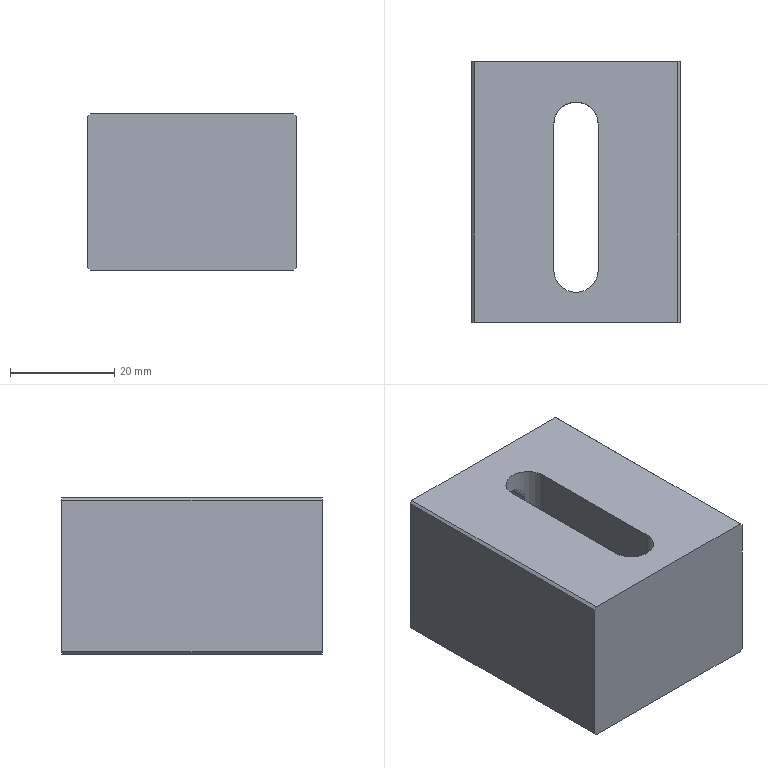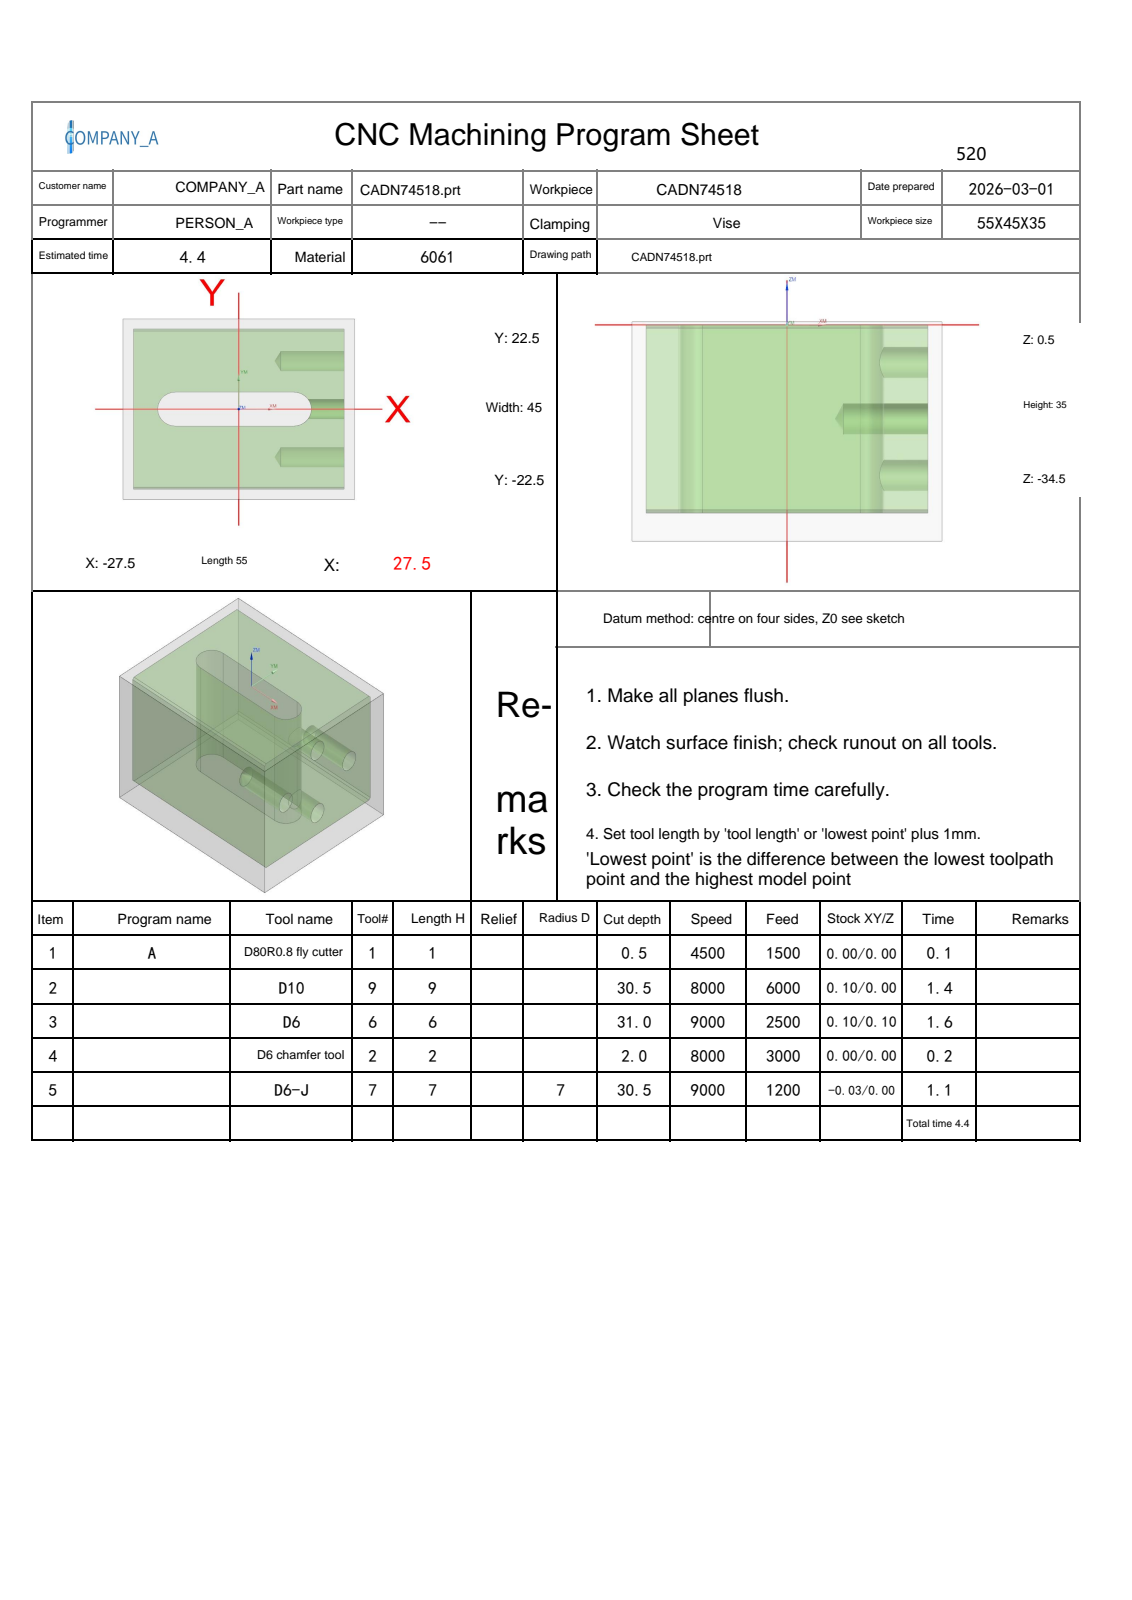NC program | NX | posted by the shop | part box 40 x 50 x 30 mm
Whole program:
%
O0001
(Machine time: 5.44 MIN)
(===Total Tool:5===)
(T1=D80R0.8 fly cutter D=80.  R=0.8  D-  H01 Z=-0.   )
(T9=D10     D=10.  R=0.   D-  H09 Z=-30.  )
(T6=D6      D=6.   R=0.   D-  H06 Z=-30.5 )
(T2=D6 chamfer tool   D=6.   R=0.   D-  H02 Z=-1.5  )
(T7=D6-J    D=6.   R=0.   D7  H07 Z=-30.  )
G80 G90 G17 G49 G40
G91 G28 Z0
M01
N1 T01 M06
(D80R0.8 fly cutter D=80. R=0.8 H=01 ce=0.00 di=0.00)
G00 G90 G54 X-70. Y0.0 M03 S4500
G43 H01 Z50.
M08
Z2.
G01 Z0.0 F1500.
X-65.
X65.
X70.
Z2.
G00 Z50.
G91 G28 Z0.0
M05
M09
G91 G28 Z0.0
M01
N2 T09 M06
(D10  D=10. R=0. H=09 ce=0.10 di=0.00)
G00 G90 G54 X0.0 Y25.1 M03 S8000
G43 H09 Z50.
M08
Z.5
G01 X25. Z.408 F6000.
G02 X30.1 Y20. Z.378 I0.0 J-5.1
G01 Y-20. Z.231
G02 X25. Y-25.1 Z.201 I-5.1 J0.0
G01 X-25. Z.017
G02 X-30.1 Y-20. Z-.013 I0.0 J5.1
G01 Y20. Z-.16
G02 X-25. Y25.1 Z-.19 I5.1 J0.0
G01 X25. Z-.374
G02 X30.1 Y20. Z-.404 I0.0 J-5.1
G01 Y-20. Z-.551
G02 X25. Y-25.1 Z-.581 I-5.1 J0.0
G01 X-25. Z-.765
G02 X-30.1 Y-20. Z-.795 I0.0 J5.1
G01 Y20. Z-.942
G02 X-25. Y25.1 Z-.972 I5.1 J0.0
G01 X25. Z-1.156
G02 X30.1 Y20. Z-1.186 I0.0 J-5.1
G01 Y-20. Z-1.333
G02 X25. Y-25.1 Z-1.363 I-5.1 J0.0
G01 X-25. Z-1.547
G02 X-30.1 Y-20. Z-1.577 I0.0 J5.1
G01 Y20. Z-1.724
G02 X-25. Y25.1 Z-1.754 I5.1 J0.0
G01 X25. Z-1.938
G02 X30.1 Y20. Z-1.968 I0.0 J-5.1
G01 Y-20. Z-2.115
G02 X25. Y-25.1 Z-2.145 I-5.1 J0.0
G01 X-25. Z-2.329
G02 X-30.1 Y-20. Z-2.359 I0.0 J5.1
G01 Y20. Z-2.506
G02 X-25. Y25.1 Z-2.536 I5.1 J0.0
G01 X25. Z-2.72
G02 X30.1 Y20. Z-2.75 I0.0 J-5.1
G01 Y-20. Z-2.897
G02 X25. Y-25.1 Z-2.927 I-5.1 J0.0
G01 X-25. Z-3.111
G02 X-30.1 Y-20. Z-3.141 I0.0 J5.1
G01 Y20. Z-3.289
G02 X-25. Y25.1 Z-3.318 I5.1 J0.0
G01 X25. Z-3.502
G02 X30.1 Y20. Z-3.532 I0.0 J-5.1
G01 Y-20. Z-3.68
G02 X25. Y-25.1 Z-3.709 I-5.1 J0.0
G01 X-25. Z-3.893
G02 X-30.1 Y-20. Z-3.923 I0.0 J5.1
G01 Y20. Z-4.071
G02 X-25. Y25.1 Z-4.1 I5.1 J0.0
G01 X25. Z-4.285
G02 X30.1 Y20. Z-4.314 I0.0 J-5.1
G01 Y-20. Z-4.462
G02 X25. Y-25.1 Z-4.491 I-5.1 J0.0
G01 X-25. Z-4.676
G02 X-30.1 Y-20. Z-4.705 I0.0 J5.1
G01 Y20. Z-4.853
G02 X-25. Y25.1 Z-4.882 I5.1 J0.0
G01 X25. Z-5.067
G02 X30.1 Y20. Z-5.096 I0.0 J-5.1
G01 Y-20. Z-5.244
G02 X25. Y-25.1 Z-5.273 I-5.1 J0.0
G01 X-25. Z-5.458
G02 X-30.1 Y-20. Z-5.487 I0.0 J5.1
G01 Y20. Z-5.635
G02 X-25. Y25.1 Z-5.664 I5.1 J0.0
G01 X25. Z-5.849
G02 X30.1 Y20. Z-5.878 I0.0 J-5.1
G01 Y-20. Z-6.026
G02 X25. Y-25.1 Z-6.055 I-5.1 J0.0
G01 X-25. Z-6.24
G02 X-30.1 Y-20. Z-6.269 I0.0 J5.1
G01 Y20. Z-6.417
G02 X-25. Y25.1 Z-6.446 I5.1 J0.0
G01 X25. Z-6.631
G02 X30.1 Y20. Z-6.66 I0.0 J-5.1
G01 Y-20. Z-6.808
G02 X25. Y-25.1 Z-6.837 I-5.1 J0.0
G01 X-25. Z-7.022
G02 X-30.1 Y-20. Z-7.051 I0.0 J5.1
G01 Y20. Z-7.199
G02 X-25. Y25.1 Z-7.228 I5.1 J0.0
G01 X25. Z-7.413
G02 X30.1 Y20. Z-7.442 I0.0 J-5.1
G01 Y-20. Z-7.59
G02 X25. Y-25.1 Z-7.619 I-5.1 J0.0
G01 X-25. Z-7.804
G02 X-30.1 Y-20. Z-7.833 I0.0 J5.1
G01 Y20. Z-7.981
G02 X-25. Y25.1 Z-8.01 I5.1 J0.0
G01 X25. Z-8.195
G02 X30.1 Y20. Z-8.224 I0.0 J-5.1
G01 Y-20. Z-8.372
G02 X25. Y-25.1 Z-8.401 I-5.1 J0.0
G01 X-25. Z-8.586
G02 X-30.1 Y-20. Z-8.615 I0.0 J5.1
G01 Y20. Z-8.763
G02 X-25. Y25.1 Z-8.792 I5.1 J0.0
G01 X25. Z-8.977
G02 X30.1 Y20. Z-9.006 I0.0 J-5.1
G01 Y-20. Z-9.154
G02 X25. Y-25.1 Z-9.183 I-5.1 J0.0
G01 X-25. Z-9.368
G02 X-30.1 Y-20. Z-9.397 I0.0 J5.1
G01 Y20. Z-9.545
G02 X-25. Y25.1 Z-9.574 I5.1 J0.0
G01 X25. Z-9.759
G02 X30.1 Y20. Z-9.788 I0.0 J-5.1
G01 Y-20. Z-9.936
G02 X25. Y-25.1 Z-9.965 I-5.1 J0.0
G01 X-25. Z-10.15
G02 X-30.1 Y-20. Z-10.179 I0.0 J5.1
G01 Y20. Z-10.327
G02 X-25. Y25.1 Z-10.357 I5.1 J0.0
G01 X25. Z-10.541
G02 X30.1 Y20. Z-10.57 I0.0 J-5.1
G01 Y-20. Z-10.718
G02 X25. Y-25.1 Z-10.748 I-5.1 J0.0
G01 X-25. Z-10.932
G02 X-30.1 Y-20. Z-10.961 I0.0 J5.1
G01 Y20. Z-11.109
G02 X-25. Y25.1 Z-11.139 I5.1 J0.0
G01 X25. Z-11.323
G02 X30.1 Y20. Z-11.353 I0.0 J-5.1
G01 Y-20. Z-11.5
G02 X25. Y-25.1 Z-11.53 I-5.1 J0.0
G01 X-25. Z-11.714
G02 X-30.1 Y-20. Z-11.744 I0.0 J5.1
G01 Y20. Z-11.891
G02 X-25. Y25.1 Z-11.921 I5.1 J0.0
G01 X25. Z-12.105
G02 X30.1 Y20. Z-12.135 I0.0 J-5.1
G01 Y-20. Z-12.282
G02 X25. Y-25.1 Z-12.312 I-5.1 J0.0
G01 X-25. Z-12.496
G02 X-30.1 Y-20. Z-12.526 I0.0 J5.1
G01 Y20. Z-12.673
G02 X-25. Y25.1 Z-12.703 I5.1 J0.0
G01 X25. Z-12.887
G02 X30.1 Y20. Z-12.917 I0.0 J-5.1
G01 Y-20. Z-13.064
G02 X25. Y-25.1 Z-13.094 I-5.1 J0.0
G01 X-25. Z-13.278
G02 X-30.1 Y-20. Z-13.308 I0.0 J5.1
G01 Y20. Z-13.455
G02 X-25. Y25.1 Z-13.485 I5.1 J0.0
G01 X25. Z-13.669
G02 X30.1 Y20. Z-13.699 I0.0 J-5.1
G01 Y-20. Z-13.846
G02 X25. Y-25.1 Z-13.876 I-5.1 J0.0
G01 X-25. Z-14.06
G02 X-30.1 Y-20. Z-14.09 I0.0 J5.1
G01 Y20. Z-14.237
G02 X-25. Y25.1 Z-14.267 I5.1 J0.0
G01 X25. Z-14.451
G02 X30.1 Y20. Z-14.481 I0.0 J-5.1
G01 Y-20. Z-14.628
G02 X25. Y-25.1 Z-14.658 I-5.1 J0.0
G01 X-25. Z-14.842
G02 X-30.1 Y-20. Z-14.872 I0.0 J5.1
G01 Y20. Z-15.019
G02 X-25. Y25.1 Z-15.049 I5.1 J0.0
G01 X25. Z-15.233
G02 X30.1 Y20. Z-15.263 I0.0 J-5.1
G01 Y-20. Z-15.41
G02 X25. Y-25.1 Z-15.44 I-5.1 J0.0
G01 X-25. Z-15.624
G02 X-30.1 Y-20. Z-15.654 I0.0 J5.1
G01 Y20. Z-15.801
G02 X-25. Y25.1 Z-15.831 I5.1 J0.0
G01 X25. Z-16.015
G02 X30.1 Y20. Z-16.045 I0.0 J-5.1
G01 Y-20. Z-16.192
G02 X25. Y-25.1 Z-16.222 I-5.1 J0.0
G01 X-25. Z-16.406
G02 X-30.1 Y-20. Z-16.436 I0.0 J5.1
G01 Y20. Z-16.583
G02 X-25. Y25.1 Z-16.613 I5.1 J0.0
G01 X25. Z-16.797
G02 X30.1 Y20. Z-16.827 I0.0 J-5.1
G01 Y-20. Z-16.974
G02 X25. Y-25.1 Z-17.004 I-5.1 J0.0
G01 X-25. Z-17.188
G02 X-30.1 Y-20. Z-17.218 I0.0 J5.1
G01 Y20. Z-17.365
G02 X-25. Y25.1 Z-17.395 I5.1 J0.0
G01 X25. Z-17.579
G02 X30.1 Y20. Z-17.609 I0.0 J-5.1
G01 Y-20. Z-17.756
G02 X25. Y-25.1 Z-17.786 I-5.1 J0.0
G01 X-25. Z-17.97
G02 X-30.1 Y-20. Z-18. I0.0 J5.1
G01 Y20. Z-18.147
G02 X-25. Y25.1 Z-18.177 I5.1 J0.0
G01 X25. Z-18.361
G02 X30.1 Y20. Z-18.391 I0.0 J-5.1
G01 Y-20. Z-18.539
G02 X25. Y-25.1 Z-18.568 I-5.1 J0.0
G01 X-25. Z-18.752
G02 X-30.1 Y-20. Z-18.782 I0.0 J5.1
G01 Y20. Z-18.93
G02 X-25. Y25.1 Z-18.959 I5.1 J0.0
G01 X25. Z-19.143
G02 X30.1 Y20. Z-19.173 I0.0 J-5.1
G01 Y-20. Z-19.321
G02 X25. Y-25.1 Z-19.35 I-5.1 J0.0
G01 X-25. Z-19.535
G02 X-30.1 Y-20. Z-19.564 I0.0 J5.1
G01 Y20. Z-19.712
G02 X-25. Y25.1 Z-19.741 I5.1 J0.0
G01 X25. Z-19.926
G02 X30.1 Y20. Z-19.955 I0.0 J-5.1
G01 Y-20. Z-20.103
G02 X25. Y-25.1 Z-20.132 I-5.1 J0.0
G01 X-25. Z-20.317
G02 X-30.1 Y-20. Z-20.346 I0.0 J5.1
G01 Y20. Z-20.494
G02 X-25. Y25.1 Z-20.523 I5.1 J0.0
G01 X25. Z-20.708
G02 X30.1 Y20. Z-20.737 I0.0 J-5.1
G01 Y-20. Z-20.885
G02 X25. Y-25.1 Z-20.914 I-5.1 J0.0
G01 X-25. Z-21.099
G02 X-30.1 Y-20. Z-21.128 I0.0 J5.1
G01 Y20. Z-21.276
G02 X-25. Y25.1 Z-21.305 I5.1 J0.0
G01 X25. Z-21.49
G02 X30.1 Y20. Z-21.519 I0.0 J-5.1
G01 Y-20. Z-21.667
G02 X25. Y-25.1 Z-21.696 I-5.1 J0.0
G01 X-25. Z-21.881
G02 X-30.1 Y-20. Z-21.91 I0.0 J5.1
G01 Y20. Z-22.058
G02 X-25. Y25.1 Z-22.087 I5.1 J0.0
G01 X25. Z-22.272
G02 X30.1 Y20. Z-22.301 I0.0 J-5.1
G01 Y-20. Z-22.449
G02 X25. Y-25.1 Z-22.478 I-5.1 J0.0
G01 X-25. Z-22.663
G02 X-30.1 Y-20. Z-22.692 I0.0 J5.1
G01 Y20. Z-22.84
G02 X-25. Y25.1 Z-22.869 I5.1 J0.0
G01 X25. Z-23.054
G02 X30.1 Y20. Z-23.083 I0.0 J-5.1
G01 Y-20. Z-23.231
G02 X25. Y-25.1 Z-23.26 I-5.1 J0.0
G01 X-25. Z-23.445
G02 X-30.1 Y-20. Z-23.474 I0.0 J5.1
G01 Y20. Z-23.622
G02 X-25. Y25.1 Z-23.651 I5.1 J0.0
G01 X25. Z-23.836
G02 X30.1 Y20. Z-23.865 I0.0 J-5.1
G01 Y-20. Z-24.013
G02 X25. Y-25.1 Z-24.042 I-5.1 J0.0
G01 X-25. Z-24.227
G02 X-30.1 Y-20. Z-24.256 I0.0 J5.1
G01 Y20. Z-24.404
G02 X-25. Y25.1 Z-24.433 I5.1 J0.0
G01 X25. Z-24.618
G02 X30.1 Y20. Z-24.647 I0.0 J-5.1
G01 Y-20. Z-24.795
G02 X25. Y-25.1 Z-24.824 I-5.1 J0.0
G01 X-25. Z-25.009
G02 X-30.1 Y-20. Z-25.038 I0.0 J5.1
G01 Y20. Z-25.186
G02 X-25. Y25.1 Z-25.215 I5.1 J0.0
G01 X25. Z-25.4
G02 X30.1 Y20. Z-25.429 I0.0 J-5.1
G01 Y-20. Z-25.577
G02 X25. Y-25.1 Z-25.607 I-5.1 J0.0
G01 X-25. Z-25.791
G02 X-30.1 Y-20. Z-25.82 I0.0 J5.1
G01 Y20. Z-25.968
G02 X-25. Y25.1 Z-25.998 I5.1 J0.0
G01 X25. Z-26.182
G02 X30.1 Y20. Z-26.211 I0.0 J-5.1
G01 Y-20. Z-26.359
G02 X25. Y-25.1 Z-26.389 I-5.1 J0.0
G01 X-25. Z-26.573
G02 X-30.1 Y-20. Z-26.603 I0.0 J5.1
G01 Y20. Z-26.75
G02 X-25. Y25.1 Z-26.78 I5.1 J0.0
G01 X25. Z-26.964
G02 X30.1 Y20. Z-26.994 I0.0 J-5.1
G01 Y-20. Z-27.141
G02 X25. Y-25.1 Z-27.171 I-5.1 J0.0
G01 X-25. Z-27.355
G02 X-30.1 Y-20. Z-27.385 I0.0 J5.1
G01 Y20. Z-27.532
G02 X-25. Y25.1 Z-27.562 I5.1 J0.0
G01 X25. Z-27.746
G02 X30.1 Y20. Z-27.776 I0.0 J-5.1
G01 Y-20. Z-27.923
G02 X25. Y-25.1 Z-27.953 I-5.1 J0.0
G01 X-25. Z-28.137
G02 X-30.1 Y-20. Z-28.167 I0.0 J5.1
G01 Y20. Z-28.314
G02 X-25. Y25.1 Z-28.344 I5.1 J0.0
G01 X25. Z-28.528
G02 X30.1 Y20. Z-28.558 I0.0 J-5.1
G01 Y-20. Z-28.705
G02 X25. Y-25.1 Z-28.735 I-5.1 J0.0
G01 X-25. Z-28.919
G02 X-30.1 Y-20. Z-28.949 I0.0 J5.1
G01 Y20. Z-29.096
G02 X-25. Y25.1 Z-29.126 I5.1 J0.0
G01 X25. Z-29.31
G02 X30.1 Y20. Z-29.34 I0.0 J-5.1
G01 Y-20. Z-29.487
G02 X25. Y-25.1 Z-29.517 I-5.1 J0.0
G01 X-25. Z-29.701
G02 X-30.1 Y-20. Z-29.731 I0.0 J5.1
G01 Y20. Z-29.878
G02 X-25. Y25.1 Z-29.908 I5.1 J0.0
G01 X0.0 Z-30.
X25.
G02 X30.1 Y20. I0.0 J-5.1
G01 Y-20.
G02 X25. Y-25.1 I-5.1 J0.0
G01 X-25.
G02 X-30.1 Y-20. I0.0 J5.1
G01 Y20.
G02 X-25. Y25.1 I5.1 J0.0
G01 X0.0
X.5
Z-29.
G00 Z50.
G91 G28 Z0.0
M05
M09
G91 G28 Z0.0
M01
N3 T06 M06
(D6  D=6. R=0. H=06 ce=0.10 di=0.10)
G00 G90 G54 X-1. Y1.15 M03 S9000
G43 H06 Z50.
M08
Z.5
G01 X-15. Z.389 F2500.
G03 X-16.15 Y0.0 Z.375 I0.0 J-1.15
X-15. Y-1.15 Z.361 I1.15 J0.0
G01 X13. Z.139
G03 X14.15 Y0.0 Z.125 I0.0 J1.15
X13. Y1.15 Z.111 I-1.15 J0.0
G01 X-15. Z-.111
G03 X-16.15 Y0.0 Z-.125 I0.0 J-1.15
X-15. Y-1.15 Z-.139 I1.15 J0.0
G01 X13. Z-.361
G03 X14.15 Y0.0 Z-.375 I0.0 J1.15
X13. Y1.15 Z-.389 I-1.15 J0.0
G01 X-15. Z-.611
G03 X-16.15 Y0.0 Z-.625 I0.0 J-1.15
X-15. Y-1.15 Z-.639 I1.15 J0.0
G01 X13. Z-.861
G03 X14.15 Y0.0 Z-.875 I0.0 J1.15
X13. Y1.15 Z-.889 I-1.15 J0.0
G01 X-15. Z-1.111
G03 X-16.15 Y0.0 Z-1.125 I0.0 J-1.15
X-15. Y-1.15 Z-1.139 I1.15 J0.0
G01 X13. Z-1.361
G03 X14.15 Y0.0 Z-1.375 I0.0 J1.15
X13. Y1.15 Z-1.389 I-1.15 J0.0
G01 X-15. Z-1.611
G03 X-16.15 Y0.0 Z-1.625 I0.0 J-1.15
X-15. Y-1.15 Z-1.639 I1.15 J0.0
G01 X13. Z-1.861
G03 X14.15 Y0.0 Z-1.875 I0.0 J1.15
X13. Y1.15 Z-1.889 I-1.15 J0.0
G01 X-15. Z-2.111
G03 X-16.15 Y0.0 Z-2.125 I0.0 J-1.15
X-15. Y-1.15 Z-2.139 I1.15 J0.0
G01 X13. Z-2.361
G03 X14.15 Y0.0 Z-2.375 I0.0 J1.15
X13. Y1.15 Z-2.389 I-1.15 J0.0
G01 X-15. Z-2.611
G03 X-16.15 Y0.0 Z-2.625 I0.0 J-1.15
X-15. Y-1.15 Z-2.639 I1.15 J0.0
G01 X13. Z-2.861
G03 X14.15 Y0.0 Z-2.875 I0.0 J1.15
X13. Y1.15 Z-2.889 I-1.15 J0.0
G01 X-15. Z-3.111
G03 X-16.15 Y0.0 Z-3.125 I0.0 J-1.15
X-15. Y-1.15 Z-3.139 I1.15 J0.0
G01 X13. Z-3.361
G03 X14.15 Y0.0 Z-3.375 I0.0 J1.15
X13. Y1.15 Z-3.389 I-1.15 J0.0
G01 X-15. Z-3.611
G03 X-16.15 Y0.0 Z-3.625 I0.0 J-1.15
X-15. Y-1.15 Z-3.639 I1.15 J0.0
G01 X13. Z-3.861
G03 X14.15 Y0.0 Z-3.875 I0.0 J1.15
X13. Y1.15 Z-3.889 I-1.15 J0.0
G01 X-15. Z-4.111
G03 X-16.15 Y0.0 Z-4.125 I0.0 J-1.15
X-15. Y-1.15 Z-4.139 I1.15 J0.0
G01 X13. Z-4.361
G03 X14.15 Y0.0 Z-4.375 I0.0 J1.15
X13. Y1.15 Z-4.389 I-1.15 J0.0
G01 X-15. Z-4.611
G03 X-16.15 Y0.0 Z-4.625 I0.0 J-1.15
X-15. Y-1.15 Z-4.639 I1.15 J0.0
G01 X13. Z-4.861
G03 X14.15 Y0.0 Z-4.875 I0.0 J1.15
X13. Y1.15 Z-4.889 I-1.15 J0.0
G01 X-15. Z-5.111
G03 X-16.15 Y0.0 Z-5.125 I0.0 J-1.15
X-15. Y-1.15 Z-5.139 I1.15 J0.0
G01 X13. Z-5.361
G03 X14.15 Y0.0 Z-5.375 I0.0 J1.15
X13. Y1.15 Z-5.389 I-1.15 J0.0
G01 X-15. Z-5.611
G03 X-16.15 Y0.0 Z-5.625 I0.0 J-1.15
X-15. Y-1.15 Z-5.639 I1.15 J0.0
G01 X13. Z-5.861
G03 X14.15 Y0.0 Z-5.875 I0.0 J1.15
X13. Y1.15 Z-5.889 I-1.15 J0.0
G01 X-15. Z-6.111
G03 X-16.15 Y0.0 Z-6.125 I0.0 J-1.15
X-15. Y-1.15 Z-6.139 I1.15 J0.0
G01 X13. Z-6.361
G03 X14.15 Y0.0 Z-6.375 I0.0 J1.15
X13. Y1.15 Z-6.389 I-1.15 J0.0
G01 X-15. Z-6.611
G03 X-16.15 Y0.0 Z-6.625 I0.0 J-1.15
X-15. Y-1.15 Z-6.639 I1.15 J0.0
G01 X13. Z-6.861
G03 X14.15 Y0.0 Z-6.875 I0.0 J1.15
X13. Y1.15 Z-6.889 I-1.15 J0.0
G01 X-15. Z-7.111
G03 X-16.15 Y0.0 Z-7.125 I0.0 J-1.15
X-15. Y-1.15 Z-7.139 I1.15 J0.0
G01 X13. Z-7.361
G03 X14.15 Y0.0 Z-7.375 I0.0 J1.15
X13. Y1.15 Z-7.389 I-1.15 J0.0
G01 X-15. Z-7.611
G03 X-16.15 Y0.0 Z-7.625 I0.0 J-1.15
X-15. Y-1.15 Z-7.639 I1.15 J0.0
G01 X13. Z-7.861
G03 X14.15 Y0.0 Z-7.875 I0.0 J1.15
X13. Y1.15 Z-7.889 I-1.15 J0.0
G01 X-15. Z-8.111
G03 X-16.15 Y0.0 Z-8.125 I0.0 J-1.15
X-15. Y-1.15 Z-8.139 I1.15 J0.0
G01 X13. Z-8.361
G03 X14.15 Y0.0 Z-8.375 I0.0 J1.15
X13. Y1.15 Z-8.389 I-1.15 J0.0
G01 X-15. Z-8.611
G03 X-16.15 Y0.0 Z-8.625 I0.0 J-1.15
X-15. Y-1.15 Z-8.639 I1.15 J0.0
G01 X13. Z-8.861
G03 X14.15 Y0.0 Z-8.875 I0.0 J1.15
X13. Y1.15 Z-8.889 I-1.15 J0.0
G01 X-15. Z-9.111
G03 X-16.15 Y0.0 Z-9.125 I0.0 J-1.15
X-15. Y-1.15 Z-9.139 I1.15 J0.0
G01 X13. Z-9.361
G03 X14.15 Y0.0 Z-9.375 I0.0 J1.15
X13. Y1.15 Z-9.389 I-1.15 J0.0
G01 X-15. Z-9.611
G03 X-16.15 Y0.0 Z-9.625 I0.0 J-1.15
X-15. Y-1.15 Z-9.639 I1.15 J0.0
G01 X13. Z-9.861
G03 X14.15 Y0.0 Z-9.875 I0.0 J1.15
X13. Y1.15 Z-9.889 I-1.15 J0.0
G01 X-15. Z-10.111
G03 X-16.15 Y0.0 Z-10.125 I0.0 J-1.15
X-15. Y-1.15 Z-10.139 I1.15 J0.0
G01 X13. Z-10.361
G03 X14.15 Y0.0 Z-10.375 I0.0 J1.15
X13. Y1.15 Z-10.389 I-1.15 J0.0
G01 X-15. Z-10.611
G03 X-16.15 Y0.0 Z-10.625 I0.0 J-1.15
X-15. Y-1.15 Z-10.639 I1.15 J0.0
G01 X13. Z-10.861
G03 X14.15 Y0.0 Z-10.875 I0.0 J1.15
X13. Y1.15 Z-10.889 I-1.15 J0.0
G01 X-15. Z-11.111
G03 X-16.15 Y0.0 Z-11.125 I0.0 J-1.15
X-15. Y-1.15 Z-11.139 I1.15 J0.0
G01 X13. Z-11.361
G03 X14.15 Y0.0 Z-11.375 I0.0 J1.15
X13. Y1.15 Z-11.389 I-1.15 J0.0
G01 X-15. Z-11.611
G03 X-16.15 Y0.0 Z-11.625 I0.0 J-1.15
X-15. Y-1.15 Z-11.639 I1.15 J0.0
G01 X13. Z-11.861
G03 X14.15 Y0.0 Z-11.875 I0.0 J1.15
X13. Y1.15 Z-11.889 I-1.15 J0.0
G01 X-15. Z-12.111
G03 X-16.15 Y0.0 Z-12.125 I0.0 J-1.15
X-15. Y-1.15 Z-12.139 I1.15 J0.0
G01 X13. Z-12.361
G03 X14.15 Y0.0 Z-12.375 I0.0 J1.15
X13. Y1.15 Z-12.389 I-1.15 J0.0
G01 X-15. Z-12.611
G03 X-16.15 Y0.0 Z-12.625 I0.0 J-1.15
X-15. Y-1.15 Z-12.639 I1.15 J0.0
G01 X13. Z-12.861
G03 X14.15 Y0.0 Z-12.875 I0.0 J1.15
X13. Y1.15 Z-12.889 I-1.15 J0.0
G01 X-15. Z-13.111
G03 X-16.15 Y0.0 Z-13.125 I0.0 J-1.15
X-15. Y-1.15 Z-13.139 I1.15 J0.0
G01 X13. Z-13.361
G03 X14.15 Y0.0 Z-13.375 I0.0 J1.15
X13. Y1.15 Z-13.389 I-1.15 J0.0
G01 X-15. Z-13.611
G03 X-16.15 Y0.0 Z-13.625 I0.0 J-1.15
X-15. Y-1.15 Z-13.639 I1.15 J0.0
G01 X13. Z-13.861
G03 X14.15 Y0.0 Z-13.875 I0.0 J1.15
X13. Y1.15 Z-13.889 I-1.15 J0.0
G01 X-15. Z-14.111
G03 X-16.15 Y0.0 Z-14.125 I0.0 J-1.15
X-15. Y-1.15 Z-14.139 I1.15 J0.0
G01 X13. Z-14.361
G03 X14.15 Y0.0 Z-14.375 I0.0 J1.15
X13. Y1.15 Z-14.389 I-1.15 J0.0
G01 X-15. Z-14.611
G03 X-16.15 Y0.0 Z-14.625 I0.0 J-1.15
X-15. Y-1.15 Z-14.639 I1.15 J0.0
G01 X13. Z-14.861
G03 X14.15 Y0.0 Z-14.875 I0.0 J1.15
X13. Y1.15 Z-14.889 I-1.15 J0.0
G01 X-15. Z-15.111
G03 X-16.15 Y0.0 Z-15.125 I0.0 J-1.15
X-15. Y-1.15 Z-15.139 I1.15 J0.0
G01 X13. Z-15.361
G03 X14.15 Y0.0 Z-15.375 I0.0 J1.15
X13. Y1.15 Z-15.389 I-1.15 J0.0
G01 X-15. Z-15.611
G03 X-16.15 Y0.0 Z-15.625 I0.0 J-1.15
X-15. Y-1.15 Z-15.639 I1.15 J0.0
G01 X13. Z-15.861
G03 X14.15 Y0.0 Z-15.875 I0.0 J1.15
X13. Y1.15 Z-15.889 I-1.15 J0.0
G01 X-15. Z-16.111
G03 X-16.15 Y0.0 Z-16.125 I0.0 J-1.15
X-15. Y-1.15 Z-16.139 I1.15 J0.0
G01 X13. Z-16.361
G03 X14.15 Y0.0 Z-16.375 I0.0 J1.15
X13. Y1.15 Z-16.389 I-1.15 J0.0
G01 X-15. Z-16.611
G03 X-16.15 Y0.0 Z-16.625 I0.0 J-1.15
X-15. Y-1.15 Z-16.639 I1.15 J0.0
G01 X13. Z-16.861
G03 X14.15 Y0.0 Z-16.875 I0.0 J1.15
X13. Y1.15 Z-16.889 I-1.15 J0.0
G01 X-15. Z-17.111
G03 X-16.15 Y0.0 Z-17.125 I0.0 J-1.15
X-15. Y-1.15 Z-17.139 I1.15 J0.0
G01 X13. Z-17.361
G03 X14.15 Y0.0 Z-17.375 I0.0 J1.15
X13. Y1.15 Z-17.389 I-1.15 J0.0
G01 X-15. Z-17.611
G03 X-16.15 Y0.0 Z-17.625 I0.0 J-1.15
X-15. Y-1.15 Z-17.639 I1.15 J0.0
G01 X13. Z-17.861
G03 X14.15 Y0.0 Z-17.875 I0.0 J1.15
X13. Y1.15 Z-17.889 I-1.15 J0.0
G01 X-15. Z-18.111
G03 X-16.15 Y0.0 Z-18.125 I0.0 J-1.15
X-15. Y-1.15 Z-18.139 I1.15 J0.0
G01 X13. Z-18.361
G03 X14.15 Y0.0 Z-18.375 I0.0 J1.15
X13. Y1.15 Z-18.389 I-1.15 J0.0
G01 X-15. Z-18.611
G03 X-16.15 Y0.0 Z-18.625 I0.0 J-1.15
X-15. Y-1.15 Z-18.639 I1.15 J0.0
G01 X13. Z-18.861
G03 X14.15 Y0.0 Z-18.875 I0.0 J1.15
X13. Y1.15 Z-18.889 I-1.15 J0.0
G01 X-15. Z-19.111
G03 X-16.15 Y0.0 Z-19.125 I0.0 J-1.15
X-15. Y-1.15 Z-19.139 I1.15 J0.0
G01 X13. Z-19.361
G03 X14.15 Y0.0 Z-19.375 I0.0 J1.15
X13. Y1.15 Z-19.389 I-1.15 J0.0
G01 X-15. Z-19.611
G03 X-16.15 Y0.0 Z-19.625 I0.0 J-1.15
X-15. Y-1.15 Z-19.639 I1.15 J0.0
G01 X13. Z-19.861
G03 X14.15 Y0.0 Z-19.875 I0.0 J1.15
X13. Y1.15 Z-19.889 I-1.15 J0.0
G01 X-15. Z-20.111
G03 X-16.15 Y0.0 Z-20.125 I0.0 J-1.15
X-15. Y-1.15 Z-20.139 I1.15 J0.0
G01 X13. Z-20.361
G03 X14.15 Y0.0 Z-20.375 I0.0 J1.15
X13. Y1.15 Z-20.389 I-1.15 J0.0
G01 X-15. Z-20.611
G03 X-16.15 Y0.0 Z-20.625 I0.0 J-1.15
X-15. Y-1.15 Z-20.639 I1.15 J0.0
G01 X13. Z-20.861
G03 X14.15 Y0.0 Z-20.875 I0.0 J1.15
X13. Y1.15 Z-20.889 I-1.15 J0.0
G01 X-15. Z-21.111
G03 X-16.15 Y0.0 Z-21.125 I0.0 J-1.15
X-15. Y-1.15 Z-21.139 I1.15 J0.0
G01 X13. Z-21.361
G03 X14.15 Y0.0 Z-21.375 I0.0 J1.15
X13. Y1.15 Z-21.389 I-1.15 J0.0
G01 X-15. Z-21.611
G03 X-16.15 Y0.0 Z-21.625 I0.0 J-1.15
X-15. Y-1.15 Z-21.639 I1.15 J0.0
G01 X13. Z-21.861
G03 X14.15 Y0.0 Z-21.875 I0.0 J1.15
X13. Y1.15 Z-21.889 I-1.15 J0.0
G01 X-15. Z-22.111
G03 X-16.15 Y0.0 Z-22.125 I0.0 J-1.15
X-15. Y-1.15 Z-22.139 I1.15 J0.0
G01 X13. Z-22.361
G03 X14.15 Y0.0 Z-22.375 I0.0 J1.15
X13. Y1.15 Z-22.389 I-1.15 J0.0
G01 X-15. Z-22.611
G03 X-16.15 Y0.0 Z-22.625 I0.0 J-1.15
X-15. Y-1.15 Z-22.639 I1.15 J0.0
G01 X13. Z-22.861
G03 X14.15 Y0.0 Z-22.875 I0.0 J1.15
X13. Y1.15 Z-22.889 I-1.15 J0.0
G01 X-15. Z-23.111
G03 X-16.15 Y0.0 Z-23.125 I0.0 J-1.15
X-15. Y-1.15 Z-23.139 I1.15 J0.0
G01 X13. Z-23.361
G03 X14.15 Y0.0 Z-23.375 I0.0 J1.15
X13. Y1.15 Z-23.389 I-1.15 J0.0
G01 X-15. Z-23.611
G03 X-16.15 Y0.0 Z-23.625 I0.0 J-1.15
X-15. Y-1.15 Z-23.639 I1.15 J0.0
G01 X13. Z-23.861
G03 X14.15 Y0.0 Z-23.875 I0.0 J1.15
X13. Y1.15 Z-23.889 I-1.15 J0.0
G01 X-15. Z-24.111
G03 X-16.15 Y0.0 Z-24.125 I0.0 J-1.15
X-15. Y-1.15 Z-24.139 I1.15 J0.0
G01 X13. Z-24.361
G03 X14.15 Y0.0 Z-24.375 I0.0 J1.15
X13. Y1.15 Z-24.389 I-1.15 J0.0
G01 X-15. Z-24.611
G03 X-16.15 Y0.0 Z-24.625 I0.0 J-1.15
X-15. Y-1.15 Z-24.639 I1.15 J0.0
G01 X13. Z-24.861
G03 X14.15 Y0.0 Z-24.875 I0.0 J1.15
X13. Y1.15 Z-24.889 I-1.15 J0.0
G01 X-15. Z-25.111
G03 X-16.15 Y0.0 Z-25.125 I0.0 J-1.15
X-15. Y-1.15 Z-25.139 I1.15 J0.0
G01 X13. Z-25.361
G03 X14.15 Y0.0 Z-25.375 I0.0 J1.15
X13. Y1.15 Z-25.389 I-1.15 J0.0
G01 X-15. Z-25.611
G03 X-16.15 Y0.0 Z-25.625 I0.0 J-1.15
X-15. Y-1.15 Z-25.639 I1.15 J0.0
G01 X13. Z-25.861
G03 X14.15 Y0.0 Z-25.875 I0.0 J1.15
X13. Y1.15 Z-25.889 I-1.15 J0.0
G01 X-15. Z-26.111
G03 X-16.15 Y0.0 Z-26.125 I0.0 J-1.15
X-15. Y-1.15 Z-26.139 I1.15 J0.0
G01 X13. Z-26.361
G03 X14.15 Y0.0 Z-26.375 I0.0 J1.15
X13. Y1.15 Z-26.389 I-1.15 J0.0
G01 X-15. Z-26.611
G03 X-16.15 Y0.0 Z-26.625 I0.0 J-1.15
X-15. Y-1.15 Z-26.639 I1.15 J0.0
G01 X13. Z-26.861
G03 X14.15 Y0.0 Z-26.875 I0.0 J1.15
X13. Y1.15 Z-26.889 I-1.15 J0.0
G01 X-15. Z-27.111
G03 X-16.15 Y0.0 Z-27.125 I0.0 J-1.15
X-15. Y-1.15 Z-27.139 I1.15 J0.0
G01 X13. Z-27.361
G03 X14.15 Y0.0 Z-27.375 I0.0 J1.15
X13. Y1.15 Z-27.389 I-1.15 J0.0
G01 X-15. Z-27.611
G03 X-16.15 Y0.0 Z-27.625 I0.0 J-1.15
X-15. Y-1.15 Z-27.639 I1.15 J0.0
G01 X13. Z-27.861
G03 X14.15 Y0.0 Z-27.875 I0.0 J1.15
X13. Y1.15 Z-27.889 I-1.15 J0.0
G01 X-15. Z-28.111
G03 X-16.15 Y0.0 Z-28.125 I0.0 J-1.15
X-15. Y-1.15 Z-28.139 I1.15 J0.0
G01 X13. Z-28.361
G03 X14.15 Y0.0 Z-28.375 I0.0 J1.15
X13. Y1.15 Z-28.389 I-1.15 J0.0
G01 X-15. Z-28.611
G03 X-16.15 Y0.0 Z-28.625 I0.0 J-1.15
X-15. Y-1.15 Z-28.639 I1.15 J0.0
G01 X13. Z-28.861
G03 X14.15 Y0.0 Z-28.875 I0.0 J1.15
X13. Y1.15 Z-28.889 I-1.15 J0.0
G01 X-15. Z-29.111
G03 X-16.15 Y0.0 Z-29.125 I0.0 J-1.15
X-15. Y-1.15 Z-29.139 I1.15 J0.0
G01 X13. Z-29.361
G03 X14.15 Y0.0 Z-29.375 I0.0 J1.15
X13. Y1.15 Z-29.389 I-1.15 J0.0
G01 X-15. Z-29.611
G03 X-16.15 Y0.0 Z-29.625 I0.0 J-1.15
X-15. Y-1.15 Z-29.639 I1.15 J0.0
G01 X13. Z-29.861
G03 X14.15 Y0.0 Z-29.875 I0.0 J1.15
X13. Y1.15 Z-29.889 I-1.15 J0.0
G01 X-15. Z-30.111
G03 X-16.15 Y0.0 Z-30.125 I0.0 J-1.15
X-15. Y-1.15 Z-30.139 I1.15 J0.0
G01 X13. Z-30.361
G03 X14.15 Y0.0 Z-30.375 I0.0 J1.15
X13. Y1.15 Z-30.389 I-1.15 J0.0
G01 X-1. Z-30.5
X-15.
G03 X-16.15 Y0.0 I0.0 J-1.15
X-15. Y-1.15 I1.15 J0.0
G01 X13.
G03 X14.15 Y0.0 I0.0 J1.15
X13. Y1.15 I-1.15 J0.0
G01 X-1.
X-1.5
Z-29.5
G00 Z50.
G91 G28 Z0.0
M05
M09
G91 G28 Z0.0
M01
N4 T02 M06
(D6 chamfer tool D=6. R=0. H=02 ce=0.00 di=0.00)
G00 G90 G54 X26.207 Y19.961 M03 S8000
G43 H02 Z50.
M08
Z2.935
G01 Z-1.5 F3000.
X26.267 Y19.789
X26.3 Y19.5
Y-19.5
X26.267 Y-19.789
X26.207 Y-19.961
Z2.935
G00 Z50.
X-26.207
Z2.935
G01 Z-1.5
X-26.267 Y-19.789
X-26.3 Y-19.5
Y19.5
X-26.267 Y19.789
X-26.207 Y19.961
Z2.935
G00 Z50.
X-.75 Y2.122
Z2.099
G01 Z-1.5
G03 X-.67 Y2.422 I-.52 J.3
X-.97 Y2.942 I-.6 J0.0
G01 X-1. Y2.95
X-15.
G03 X-17.95 Y0.0 I0.0 J-2.95
X-15. Y-2.95 I2.95 J0.0
G01 X13.
G03 X15.95 Y0.0 I0.0 J2.95
X13. Y2.95 I-2.95 J0.0
G01 X-1.
X-1.03 Y2.942
G03 X-1.33 Y2.422 I.3 J-.52
X-1.25 Y2.122 I.6 J0.0
G01 Z2.099
G00 Z50.
G00 G90 X28.963 Y-21.9 M03 S6500
Z50.
Z.3
G01 Z-1.2 F1500.
G03 X27.763 Y-20.7 I-1.2 J0.0
G01 X-27.763
G03 X-28.963 Y-21.9 I0.0 J-1.2
G01 Z.3
G00 Z50.
Y21.9
Z.3
G01 Z-1.2
G03 X-27.763 Y20.7 I1.2 J0.0
G01 X27.763
G03 X28.963 Y21.9 I0.0 J1.2
G01 Z.3
G00 Z50.
G91 G28 Z0.0
M05
M09
G91 G28 Z0.0
M01
N5 T07 M06
(D6-J  D=6. R=0. H=07 ce=0.00 di=0.00)
G00 G90 G54 X-1.2 Y-1. M03 S8000
G43 H07 Z50.
M08
Z-5.5
G01 Z-6. F600.
G41 D07
Y-1.05
G03 X-1. Y-1.25 I.2 J0.0
G01 X13.
G03 X14.25 Y0.0 I0.0 J1.25
X13. Y1.25 I-1.25 J0.0
G01 X-15.
G03 X-16.25 Y0.0 I0.0 J-1.25
X-15. Y-1.25 I1.25 J0.0
G01 X-1.
X-.5
G03 X-.3 Y-1.05 I0.0 J.2
G01 G40 Y-1.
Z-5.5
G00 Z1.
X-1.2
Z-11.5
G01 Z-12.
G41 D07
Y-1.05
G03 X-1. Y-1.25 I.2 J0.0
G01 X13.
G03 X14.25 Y0.0 I0.0 J1.25
X13. Y1.25 I-1.25 J0.0
G01 X-15.
G03 X-16.25 Y0.0 I0.0 J-1.25
X-15. Y-1.25 I1.25 J0.0
G01 X-1.
X-.5
G03 X-.3 Y-1.05 I0.0 J.2
G01 G40 Y-1.
Z-11.5
G00 Z-5.
X-1.2
Z-17.5
G01 Z-18.
G41 D07
Y-1.05
G03 X-1. Y-1.25 I.2 J0.0
G01 X13.
G03 X14.25 Y0.0 I0.0 J1.25
X13. Y1.25 I-1.25 J0.0
G01 X-15.
G03 X-16.25 Y0.0 I0.0 J-1.25
X-15. Y-1.25 I1.25 J0.0
G01 X-1.
X-.5
G03 X-.3 Y-1.05 I0.0 J.2
G01 G40 Y-1.
Z-17.5
G00 Z-11.
X-1.2
Z-23.5
G01 Z-24.
G41 D07
Y-1.05
G03 X-1. Y-1.25 I.2 J0.0
G01 X13.
G03 X14.25 Y0.0 I0.0 J1.25
X13. Y1.25 I-1.25 J0.0
G01 X-15.
G03 X-16.25 Y0.0 I0.0 J-1.25
X-15. Y-1.25 I1.25 J0.0
G01 X-1.
X-.5
G03 X-.3 Y-1.05 I0.0 J.2
G01 G40 Y-1.
Z-23.5
G00 Z-17.
X-1.2
Z-29.5
G01 Z-30.
G41 D07
Y-1.05
G03 X-1. Y-1.25 I.2 J0.0
G01 X13.
G03 X14.25 Y0.0 I0.0 J1.25
X13. Y1.25 I-1.25 J0.0
G01 X-15.
G03 X-16.25 Y0.0 I0.0 J-1.25
X-15. Y-1.25 I1.25 J0.0
G01 X-1.
X-.5
G03 X-.3 Y-1.05 I0.0 J.2
G01 G40 Y-1.
Z-29.5
G00 Z50.
G00 G90 X26.017 Y-24.048 M03 S9000
Z50.
Z-9.5
G01 Z-10. F1200.
G41 D07
X25.992 Y-23.849
G03 X25. Y-22.975 I-.992 J-.126
G01 X-25.
G02 X-27.975 Y-20. I0.0 J2.975
G01 Y20.
G02 X-25. Y22.975 I2.975 J0.0
G01 X25.
G02 X27.975 Y20. I0.0 J-2.975
G01 Y-20.
G02 X25. Y-22.975 I-2.975 J0.0
G01 X24.5
G03 X23.5 Y-23.975 I0.0 J-1.
G01 G40 Y-24.175
Z-9.5
G00 Z50.
X26.017 Y-24.048
Z-19.5
G01 Z-20.
G41 D07
X25.992 Y-23.849
G03 X25. Y-22.975 I-.992 J-.126
G01 X-25.
G02 X-27.975 Y-20. I0.0 J2.975
G01 Y20.
G02 X-25. Y22.975 I2.975 J0.0
G01 X25.
G02 X27.975 Y20. I0.0 J-2.975
G01 Y-20.
G02 X25. Y-22.975 I-2.975 J0.0
G01 X24.5
G03 X23.5 Y-23.975 I0.0 J-1.
G01 G40 Y-24.175
Z-19.5
G00 Z50.
X26.017 Y-24.048
Z-29.5
G01 Z-30.
G41 D07
X25.992 Y-23.849
G03 X25. Y-22.975 I-.992 J-.126
G01 X-25.
G02 X-27.975 Y-20. I0.0 J2.975
G01 Y20.
G02 X-25. Y22.975 I2.975 J0.0
G01 X25.
G02 X27.975 Y20. I0.0 J-2.975
G01 Y-20.
G02 X25. Y-22.975 I-2.975 J0.0
G01 X24.5
G03 X23.5 Y-23.975 I0.0 J-1.
G01 G40 Y-24.175
Z-29.5
G00 Z50.
M05
M09
G91 G28 Z0.0
G91 G28 Y0.0
M30
%